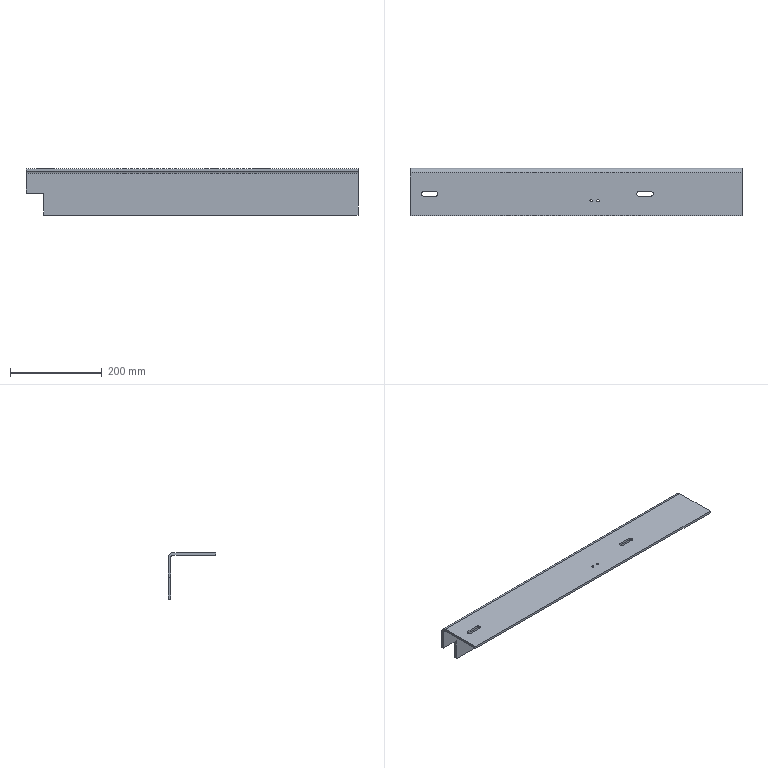Part | NX | 1 solid | 26 faces | box 724.4 x 103.1 x 101 mm | volume 696514 mm3 | plane 14 | cylinder 12 | commonest cylinder face diameters 10 x7 5 x4 20 x1
STEP:
#1=CARTESIAN_POINT('',(671.7,223.9,34.5));
#2=VERTEX_POINT('',#1);
#3=CARTESIAN_POINT('',(671.7,130.8,34.5));
#4=VERTEX_POINT('',#3);
#5=CARTESIAN_POINT('',(671.7,319.307,34.5));
#6=DIRECTION('',(0.,-1.,0.));
#7=VECTOR('',#6,1000.);
#8=LINE('',#5,#7);
#9=EDGE_CURVE('',#2,#4,#8,.T.);
#10=ORIENTED_EDGE('',*,*,#9,.T.);
#11=CARTESIAN_POINT('',(671.7,130.8,29.5));
#12=VERTEX_POINT('',#11);
#13=CARTESIAN_POINT('',(671.7,130.8,29.5));
#14=DIRECTION('',(0.,0.,1.));
#15=VECTOR('',#14,1000.);
#16=LINE('',#13,#15);
#17=EDGE_CURVE('',#12,#4,#16,.T.);
#18=ORIENTED_EDGE('',*,*,#17,.F.);
#19=CARTESIAN_POINT('',(671.7,223.9,29.5));
#20=VERTEX_POINT('',#19);
#21=CARTESIAN_POINT('',(671.7,141.246,29.5));
#22=DIRECTION('',(0.,1.,0.));
#23=VECTOR('',#22,1000.);
#24=LINE('',#21,#23);
#25=EDGE_CURVE('',#12,#20,#24,.T.);
#26=ORIENTED_EDGE('',*,*,#25,.T.);
#27=CARTESIAN_POINT('',(671.7,228.9,24.5));
#28=VERTEX_POINT('',#27);
#29=CARTESIAN_POINT('',(671.7,223.9,24.5));
#30=DIRECTION('',(-1.,0.,0.));
#31=DIRECTION('',(0.,0.,1.));
#32=AXIS2_PLACEMENT_3D('',#29,#30,#31);
#33=CIRCLE('',#32,5.);
#34=EDGE_CURVE('',#20,#28,#33,.T.);
#35=ORIENTED_EDGE('',*,*,#34,.T.);
#36=CARTESIAN_POINT('',(671.7,228.9,-66.5));
#37=VERTEX_POINT('',#36);
#38=CARTESIAN_POINT('',(671.7,228.9,29.5));
#39=DIRECTION('',(0.,0.,-1.));
#40=VECTOR('',#39,1000.);
#41=LINE('',#38,#40);
#42=EDGE_CURVE('',#28,#37,#41,.T.);
#43=ORIENTED_EDGE('',*,*,#42,.T.);
#44=CARTESIAN_POINT('',(671.7,233.9,-66.5));
#45=VERTEX_POINT('',#44);
#46=CARTESIAN_POINT('',(671.7,141.246,-66.5));
#47=DIRECTION('',(0.,1.,0.));
#48=VECTOR('',#47,1000.);
#49=LINE('',#46,#48);
#50=EDGE_CURVE('',#37,#45,#49,.T.);
#51=ORIENTED_EDGE('',*,*,#50,.T.);
#52=CARTESIAN_POINT('',(671.7,233.9,24.5));
#53=VERTEX_POINT('',#52);
#54=CARTESIAN_POINT('',(671.7,233.9,29.5));
#55=DIRECTION('',(0.,0.,1.));
#56=VECTOR('',#55,1000.);
#57=LINE('',#54,#56);
#58=EDGE_CURVE('',#45,#53,#57,.T.);
#59=ORIENTED_EDGE('',*,*,#58,.T.);
#60=CARTESIAN_POINT('',(671.7,223.9,24.5));
#61=DIRECTION('',(1.,0.,0.));
#62=DIRECTION('',(0.,1.,0.));
#63=AXIS2_PLACEMENT_3D('',#60,#61,#62);
#64=CIRCLE('',#63,10.);
#65=EDGE_CURVE('',#53,#2,#64,.T.);
#66=ORIENTED_EDGE('',*,*,#65,.T.);
#67=EDGE_LOOP('',(#10,#18,#26,#35,#43,#51,#59,#66));
#68=FACE_BOUND('',#67,.T.);
#69=CARTESIAN_POINT('',(671.7,165.9,29.5));
#70=DIRECTION('',(1.,0.,0.));
#71=DIRECTION('',(0.,1.,0.));
#72=AXIS2_PLACEMENT_3D('',#69,#70,#71);
#73=PLANE('',#72);
#74=ADVANCED_FACE('',(#68),#73,.T.);
#75=CARTESIAN_POINT('',(-52.7,130.8,29.5));
#76=VERTEX_POINT('',#75);
#77=CARTESIAN_POINT('',(357.184,130.8,29.5));
#78=DIRECTION('',(1.,0.,0.));
#79=VECTOR('',#78,1000.);
#80=LINE('',#77,#79);
#81=EDGE_CURVE('',#76,#12,#80,.T.);
#82=ORIENTED_EDGE('',*,*,#81,.T.);
#83=ORIENTED_EDGE('',*,*,#17,.T.);
#84=CARTESIAN_POINT('',(-52.7,130.8,34.5));
#85=VERTEX_POINT('',#84);
#86=CARTESIAN_POINT('',(357.184,130.8,34.5));
#87=DIRECTION('',(1.,0.,0.));
#88=VECTOR('',#87,1000.);
#89=LINE('',#86,#88);
#90=EDGE_CURVE('',#85,#4,#89,.T.);
#91=ORIENTED_EDGE('',*,*,#90,.F.);
#92=CARTESIAN_POINT('',(-52.7,130.8,29.5));
#93=DIRECTION('',(0.,0.,-1.));
#94=VECTOR('',#93,1000.);
#95=LINE('',#92,#94);
#96=EDGE_CURVE('',#85,#76,#95,.T.);
#97=ORIENTED_EDGE('',*,*,#96,.T.);
#98=EDGE_LOOP('',(#82,#83,#91,#97));
#99=FACE_BOUND('',#98,.T.);
#100=CARTESIAN_POINT('',(364.7,130.8,29.5));
#101=DIRECTION('',(0.,-1.,0.));
#102=DIRECTION('',(0.,0.,-1.));
#103=AXIS2_PLACEMENT_3D('',#100,#101,#102);
#104=PLANE('',#103);
#105=ADVANCED_FACE('',(#99),#104,.T.);
#106=ORIENTED_EDGE('',*,*,#9,.F.);
#107=CARTESIAN_POINT('',(-52.7,223.9,34.5));
#108=VERTEX_POINT('',#107);
#109=CARTESIAN_POINT('',(357.184,223.9,34.5));
#110=DIRECTION('',(1.,0.,0.));
#111=VECTOR('',#110,1000.);
#112=LINE('',#109,#111);
#113=EDGE_CURVE('',#108,#2,#112,.T.);
#114=ORIENTED_EDGE('',*,*,#113,.F.);
#115=CARTESIAN_POINT('',(-52.7,233.9,34.5));
#116=DIRECTION('',(0.,1.,0.));
#117=VECTOR('',#116,1000.);
#118=LINE('',#115,#117);
#119=EDGE_CURVE('',#85,#108,#118,.T.);
#120=ORIENTED_EDGE('',*,*,#119,.F.);
#121=ORIENTED_EDGE('',*,*,#90,.T.);
#122=EDGE_LOOP('',(#106,#114,#120,#121));
#123=FACE_BOUND('',#122,.T.);
#124=CARTESIAN_POINT('',(340.,163.7,34.5));
#125=VERTEX_POINT('',#124);
#126=CARTESIAN_POINT('',(345.,163.7,34.5));
#127=VERTEX_POINT('',#126);
#128=CARTESIAN_POINT('',(342.5,163.7,34.5));
#129=DIRECTION('',(0.,0.,1.));
#130=DIRECTION('',(1.,0.,0.));
#131=AXIS2_PLACEMENT_3D('',#128,#129,#130);
#132=CIRCLE('',#131,2.5);
#133=EDGE_CURVE('',#125,#127,#132,.T.);
#134=ORIENTED_EDGE('',*,*,#133,.F.);
#135=CARTESIAN_POINT('',(342.5,163.7,34.5));
#136=DIRECTION('',(0.,0.,1.));
#137=DIRECTION('',(1.,0.,0.));
#138=AXIS2_PLACEMENT_3D('',#135,#136,#137);
#139=CIRCLE('',#138,2.5);
#140=EDGE_CURVE('',#127,#125,#139,.T.);
#141=ORIENTED_EDGE('',*,*,#140,.F.);
#142=EDGE_LOOP('',(#134,#141));
#143=FACE_BOUND('',#142,.T.);
#144=CARTESIAN_POINT('',(355.,163.7,34.5));
#145=VERTEX_POINT('',#144);
#146=CARTESIAN_POINT('',(360.,163.7,34.5));
#147=VERTEX_POINT('',#146);
#148=CARTESIAN_POINT('',(357.5,163.7,34.5));
#149=DIRECTION('',(0.,0.,1.));
#150=DIRECTION('',(1.,0.,0.));
#151=AXIS2_PLACEMENT_3D('',#148,#149,#150);
#152=CIRCLE('',#151,2.5);
#153=EDGE_CURVE('',#145,#147,#152,.T.);
#154=ORIENTED_EDGE('',*,*,#153,.F.);
#155=CARTESIAN_POINT('',(357.5,163.7,34.5));
#156=DIRECTION('',(0.,0.,1.));
#157=DIRECTION('',(1.,0.,0.));
#158=AXIS2_PLACEMENT_3D('',#155,#156,#157);
#159=CIRCLE('',#158,2.5);
#160=EDGE_CURVE('',#147,#145,#159,.T.);
#161=ORIENTED_EDGE('',*,*,#160,.F.);
#162=EDGE_LOOP('',(#154,#161));
#163=FACE_BOUND('',#162,.T.);
#164=CARTESIAN_POINT('',(3.125,173.2,34.5));
#165=VERTEX_POINT('',#164);
#166=CARTESIAN_POINT('',(8.125,178.2,34.5));
#167=VERTEX_POINT('',#166);
#168=CARTESIAN_POINT('',(3.125,178.2,34.5));
#169=DIRECTION('',(0.,0.,1.));
#170=DIRECTION('',(1.,0.,0.));
#171=AXIS2_PLACEMENT_3D('',#168,#169,#170);
#172=CIRCLE('',#171,5.);
#173=EDGE_CURVE('',#165,#167,#172,.T.);
#174=ORIENTED_EDGE('',*,*,#173,.F.);
#175=CARTESIAN_POINT('',(-23.125,173.2,34.5));
#176=VERTEX_POINT('',#175);
#177=CARTESIAN_POINT('',(357.184,173.2,34.5));
#178=DIRECTION('',(1.,0.,0.));
#179=VECTOR('',#178,1000.);
#180=LINE('',#177,#179);
#181=EDGE_CURVE('',#176,#165,#180,.T.);
#182=ORIENTED_EDGE('',*,*,#181,.F.);
#183=CARTESIAN_POINT('',(-23.125,183.2,34.5));
#184=VERTEX_POINT('',#183);
#185=CARTESIAN_POINT('',(-23.125,178.2,34.5));
#186=DIRECTION('',(0.,0.,1.));
#187=DIRECTION('',(1.,0.,0.));
#188=AXIS2_PLACEMENT_3D('',#185,#186,#187);
#189=CIRCLE('',#188,5.);
#190=EDGE_CURVE('',#184,#176,#189,.T.);
#191=ORIENTED_EDGE('',*,*,#190,.F.);
#192=CARTESIAN_POINT('',(3.125,183.2,34.5));
#193=VERTEX_POINT('',#192);
#194=CARTESIAN_POINT('',(357.184,183.2,34.5));
#195=DIRECTION('',(-1.,0.,0.));
#196=VECTOR('',#195,1000.);
#197=LINE('',#194,#196);
#198=EDGE_CURVE('',#193,#184,#197,.T.);
#199=ORIENTED_EDGE('',*,*,#198,.F.);
#200=CARTESIAN_POINT('',(3.125,178.2,34.5));
#201=DIRECTION('',(0.,0.,1.));
#202=DIRECTION('',(1.,0.,0.));
#203=AXIS2_PLACEMENT_3D('',#200,#201,#202);
#204=CIRCLE('',#203,5.);
#205=EDGE_CURVE('',#167,#193,#204,.T.);
#206=ORIENTED_EDGE('',*,*,#205,.F.);
#207=EDGE_LOOP('',(#174,#182,#191,#199,#206));
#208=FACE_BOUND('',#207,.T.);
#209=CARTESIAN_POINT('',(473.125,173.2,34.5));
#210=VERTEX_POINT('',#209);
#211=CARTESIAN_POINT('',(478.125,178.2,34.5));
#212=VERTEX_POINT('',#211);
#213=CARTESIAN_POINT('',(473.125,178.2,34.5));
#214=DIRECTION('',(0.,0.,1.));
#215=DIRECTION('',(1.,0.,0.));
#216=AXIS2_PLACEMENT_3D('',#213,#214,#215);
#217=CIRCLE('',#216,5.);
#218=EDGE_CURVE('',#210,#212,#217,.T.);
#219=ORIENTED_EDGE('',*,*,#218,.F.);
#220=CARTESIAN_POINT('',(446.875,173.2,34.5));
#221=VERTEX_POINT('',#220);
#222=CARTESIAN_POINT('',(357.184,173.2,34.5));
#223=DIRECTION('',(1.,0.,0.));
#224=VECTOR('',#223,1000.);
#225=LINE('',#222,#224);
#226=EDGE_CURVE('',#221,#210,#225,.T.);
#227=ORIENTED_EDGE('',*,*,#226,.F.);
#228=CARTESIAN_POINT('',(446.875,183.2,34.5));
#229=VERTEX_POINT('',#228);
#230=CARTESIAN_POINT('',(446.875,178.2,34.5));
#231=DIRECTION('',(0.,0.,1.));
#232=DIRECTION('',(1.,0.,0.));
#233=AXIS2_PLACEMENT_3D('',#230,#231,#232);
#234=CIRCLE('',#233,5.);
#235=EDGE_CURVE('',#229,#221,#234,.T.);
#236=ORIENTED_EDGE('',*,*,#235,.F.);
#237=CARTESIAN_POINT('',(473.125,183.2,34.5));
#238=VERTEX_POINT('',#237);
#239=CARTESIAN_POINT('',(357.184,183.2,34.5));
#240=DIRECTION('',(-1.,0.,0.));
#241=VECTOR('',#240,1000.);
#242=LINE('',#239,#241);
#243=EDGE_CURVE('',#238,#229,#242,.T.);
#244=ORIENTED_EDGE('',*,*,#243,.F.);
#245=CARTESIAN_POINT('',(473.125,178.2,34.5));
#246=DIRECTION('',(0.,0.,1.));
#247=DIRECTION('',(1.,0.,0.));
#248=AXIS2_PLACEMENT_3D('',#245,#246,#247);
#249=CIRCLE('',#248,5.);
#250=EDGE_CURVE('',#212,#238,#249,.T.);
#251=ORIENTED_EDGE('',*,*,#250,.F.);
#252=EDGE_LOOP('',(#219,#227,#236,#244,#251));
#253=FACE_BOUND('',#252,.T.);
#254=CARTESIAN_POINT('',(-52.7,233.9,34.5));
#255=DIRECTION('',(0.,0.,1.));
#256=DIRECTION('',(1.,0.,0.));
#257=AXIS2_PLACEMENT_3D('',#254,#255,#256);
#258=PLANE('',#257);
#259=ADVANCED_FACE('',(#123,#143,#163,#208,#253),#258,.T.);
#260=CARTESIAN_POINT('',(-52.7,228.9,-18.5));
#261=VERTEX_POINT('',#260);
#262=CARTESIAN_POINT('',(-52.7,233.9,-18.5));
#263=VERTEX_POINT('',#262);
#264=CARTESIAN_POINT('',(-52.7,141.246,-18.5));
#265=DIRECTION('',(0.,1.,0.));
#266=VECTOR('',#265,1000.);
#267=LINE('',#264,#266);
#268=EDGE_CURVE('',#261,#263,#267,.T.);
#269=ORIENTED_EDGE('',*,*,#268,.F.);
#270=CARTESIAN_POINT('',(-52.7,228.9,24.5));
#271=VERTEX_POINT('',#270);
#272=CARTESIAN_POINT('',(-52.7,228.9,29.5));
#273=DIRECTION('',(0.,0.,1.));
#274=VECTOR('',#273,1000.);
#275=LINE('',#272,#274);
#276=EDGE_CURVE('',#261,#271,#275,.T.);
#277=ORIENTED_EDGE('',*,*,#276,.T.);
#278=CARTESIAN_POINT('',(-52.7,223.9,29.5));
#279=VERTEX_POINT('',#278);
#280=CARTESIAN_POINT('',(-52.7,223.9,24.5));
#281=DIRECTION('',(1.,0.,0.));
#282=DIRECTION('',(0.,1.,0.));
#283=AXIS2_PLACEMENT_3D('',#280,#281,#282);
#284=CIRCLE('',#283,5.);
#285=EDGE_CURVE('',#271,#279,#284,.T.);
#286=ORIENTED_EDGE('',*,*,#285,.T.);
#287=CARTESIAN_POINT('',(-52.7,141.246,29.5));
#288=DIRECTION('',(0.,-1.,0.));
#289=VECTOR('',#288,1000.);
#290=LINE('',#287,#289);
#291=EDGE_CURVE('',#279,#76,#290,.T.);
#292=ORIENTED_EDGE('',*,*,#291,.T.);
#293=ORIENTED_EDGE('',*,*,#96,.F.);
#294=ORIENTED_EDGE('',*,*,#119,.T.);
#295=CARTESIAN_POINT('',(-52.7,233.9,24.5));
#296=VERTEX_POINT('',#295);
#297=CARTESIAN_POINT('',(-52.7,223.9,24.5));
#298=DIRECTION('',(-1.,0.,0.));
#299=DIRECTION('',(0.,0.,1.));
#300=AXIS2_PLACEMENT_3D('',#297,#298,#299);
#301=CIRCLE('',#300,10.);
#302=EDGE_CURVE('',#108,#296,#301,.T.);
#303=ORIENTED_EDGE('',*,*,#302,.T.);
#304=CARTESIAN_POINT('',(-52.7,233.9,29.5));
#305=DIRECTION('',(0.,0.,-1.));
#306=VECTOR('',#305,1000.);
#307=LINE('',#304,#306);
#308=EDGE_CURVE('',#296,#263,#307,.T.);
#309=ORIENTED_EDGE('',*,*,#308,.T.);
#310=EDGE_LOOP('',(#269,#277,#286,#292,#293,#294,#303,#309));
#311=FACE_BOUND('',#310,.T.);
#312=CARTESIAN_POINT('',(-52.7,233.9,-60.5));
#313=DIRECTION('',(-1.,0.,0.));
#314=DIRECTION('',(0.,0.,1.));
#315=AXIS2_PLACEMENT_3D('',#312,#313,#314);
#316=PLANE('',#315);
#317=ADVANCED_FACE('',(#311),#316,.T.);
#318=CARTESIAN_POINT('',(-13.7,233.9,-66.5));
#319=VERTEX_POINT('',#318);
#320=CARTESIAN_POINT('',(-13.7,228.9,-66.5));
#321=VERTEX_POINT('',#320);
#322=CARTESIAN_POINT('',(-13.7,141.246,-66.5));
#323=DIRECTION('',(0.,-1.,0.));
#324=VECTOR('',#323,1000.);
#325=LINE('',#322,#324);
#326=EDGE_CURVE('',#319,#321,#325,.T.);
#327=ORIENTED_EDGE('',*,*,#326,.F.);
#328=CARTESIAN_POINT('',(357.184,233.9,-66.5));
#329=DIRECTION('',(-1.,0.,0.));
#330=VECTOR('',#329,1000.);
#331=LINE('',#328,#330);
#332=EDGE_CURVE('',#45,#319,#331,.T.);
#333=ORIENTED_EDGE('',*,*,#332,.F.);
#334=ORIENTED_EDGE('',*,*,#50,.F.);
#335=CARTESIAN_POINT('',(357.184,228.9,-66.5));
#336=DIRECTION('',(-1.,0.,0.));
#337=VECTOR('',#336,1000.);
#338=LINE('',#335,#337);
#339=EDGE_CURVE('',#37,#321,#338,.T.);
#340=ORIENTED_EDGE('',*,*,#339,.T.);
#341=EDGE_LOOP('',(#327,#333,#334,#340));
#342=FACE_BOUND('',#341,.T.);
#343=CARTESIAN_POINT('',(671.7,233.9,-66.5));
#344=DIRECTION('',(0.,0.,-1.));
#345=DIRECTION('',(0.,-1.,0.));
#346=AXIS2_PLACEMENT_3D('',#343,#344,#345);
#347=PLANE('',#346);
#348=ADVANCED_FACE('',(#342),#347,.T.);
#349=CARTESIAN_POINT('',(357.184,233.9,24.5));
#350=DIRECTION('',(1.,0.,0.));
#351=VECTOR('',#350,1000.);
#352=LINE('',#349,#351);
#353=EDGE_CURVE('',#296,#53,#352,.T.);
#354=ORIENTED_EDGE('',*,*,#353,.T.);
#355=ORIENTED_EDGE('',*,*,#58,.F.);
#356=ORIENTED_EDGE('',*,*,#332,.T.);
#357=CARTESIAN_POINT('',(-13.7,233.9,-18.5));
#358=VERTEX_POINT('',#357);
#359=CARTESIAN_POINT('',(-13.7,233.9,29.5));
#360=DIRECTION('',(0.,0.,-1.));
#361=VECTOR('',#360,1000.);
#362=LINE('',#359,#361);
#363=EDGE_CURVE('',#358,#319,#362,.T.);
#364=ORIENTED_EDGE('',*,*,#363,.F.);
#365=CARTESIAN_POINT('',(357.184,233.9,-18.5));
#366=DIRECTION('',(1.,0.,0.));
#367=VECTOR('',#366,1000.);
#368=LINE('',#365,#367);
#369=EDGE_CURVE('',#263,#358,#368,.T.);
#370=ORIENTED_EDGE('',*,*,#369,.F.);
#371=ORIENTED_EDGE('',*,*,#308,.F.);
#372=EDGE_LOOP('',(#354,#355,#356,#364,#370,#371));
#373=FACE_BOUND('',#372,.T.);
#374=CARTESIAN_POINT('',(-52.7,233.9,24.907));
#375=DIRECTION('',(0.,1.,0.));
#376=DIRECTION('',(1.,0.,0.));
#377=AXIS2_PLACEMENT_3D('',#374,#375,#376);
#378=PLANE('',#377);
#379=ADVANCED_FACE('',(#373),#378,.T.);
#380=ORIENTED_EDGE('',*,*,#113,.T.);
#381=ORIENTED_EDGE('',*,*,#65,.F.);
#382=ORIENTED_EDGE('',*,*,#353,.F.);
#383=ORIENTED_EDGE('',*,*,#302,.F.);
#384=EDGE_LOOP('',(#380,#381,#382,#383));
#385=FACE_BOUND('',#384,.T.);
#386=CARTESIAN_POINT('',(671.7,223.9,24.5));
#387=DIRECTION('',(1.,0.,0.));
#388=DIRECTION('',(0.,-1.,0.));
#389=AXIS2_PLACEMENT_3D('',#386,#387,#388);
#390=CYLINDRICAL_SURFACE('',#389,10.);
#391=ADVANCED_FACE('',(#385),#390,.T.);
#392=ORIENTED_EDGE('',*,*,#133,.T.);
#393=CARTESIAN_POINT('',(345.,163.7,29.5));
#394=VERTEX_POINT('',#393);
#395=CARTESIAN_POINT('',(345.,163.7,34.5));
#396=DIRECTION('',(0.,0.,1.));
#397=VECTOR('',#396,1000.);
#398=LINE('',#395,#397);
#399=EDGE_CURVE('',#394,#127,#398,.T.);
#400=ORIENTED_EDGE('',*,*,#399,.F.);
#401=CARTESIAN_POINT('',(340.,163.7,29.5));
#402=VERTEX_POINT('',#401);
#403=CARTESIAN_POINT('',(342.5,163.7,29.5));
#404=DIRECTION('',(0.,0.,1.));
#405=DIRECTION('',(1.,0.,0.));
#406=AXIS2_PLACEMENT_3D('',#403,#404,#405);
#407=CIRCLE('',#406,2.5);
#408=EDGE_CURVE('',#402,#394,#407,.T.);
#409=ORIENTED_EDGE('',*,*,#408,.F.);
#410=CARTESIAN_POINT('',(340.,163.7,34.5));
#411=DIRECTION('',(0.,0.,1.));
#412=VECTOR('',#411,1000.);
#413=LINE('',#410,#412);
#414=EDGE_CURVE('',#402,#125,#413,.T.);
#415=ORIENTED_EDGE('',*,*,#414,.T.);
#416=EDGE_LOOP('',(#392,#400,#409,#415));
#417=FACE_BOUND('',#416,.T.);
#418=CARTESIAN_POINT('',(342.5,163.7,34.5));
#419=DIRECTION('',(0.,0.,1.));
#420=DIRECTION('',(1.,0.,0.));
#421=AXIS2_PLACEMENT_3D('',#418,#419,#420);
#422=CYLINDRICAL_SURFACE('',#421,2.5);
#423=ADVANCED_FACE('',(#417),#422,.F.);
#424=CARTESIAN_POINT('',(-13.7,228.9,-18.5));
#425=VERTEX_POINT('',#424);
#426=CARTESIAN_POINT('',(357.184,228.9,-18.5));
#427=DIRECTION('',(1.,0.,0.));
#428=VECTOR('',#427,1000.);
#429=LINE('',#426,#428);
#430=EDGE_CURVE('',#261,#425,#429,.T.);
#431=ORIENTED_EDGE('',*,*,#430,.F.);
#432=ORIENTED_EDGE('',*,*,#268,.T.);
#433=ORIENTED_EDGE('',*,*,#369,.T.);
#434=CARTESIAN_POINT('',(-13.7,141.246,-18.5));
#435=DIRECTION('',(0.,1.,0.));
#436=VECTOR('',#435,1000.);
#437=LINE('',#434,#436);
#438=EDGE_CURVE('',#425,#358,#437,.T.);
#439=ORIENTED_EDGE('',*,*,#438,.F.);
#440=EDGE_LOOP('',(#431,#432,#433,#439));
#441=FACE_BOUND('',#440,.T.);
#442=CARTESIAN_POINT('',(-10.7,120.49,-18.5));
#443=DIRECTION('',(0.,0.,1.));
#444=DIRECTION('',(1.,0.,0.));
#445=AXIS2_PLACEMENT_3D('',#442,#443,#444);
#446=PLANE('',#445);
#447=ADVANCED_FACE('',(#441),#446,.F.);
#448=ORIENTED_EDGE('',*,*,#363,.T.);
#449=ORIENTED_EDGE('',*,*,#326,.T.);
#450=CARTESIAN_POINT('',(-13.7,228.9,29.5));
#451=DIRECTION('',(0.,0.,-1.));
#452=VECTOR('',#451,1000.);
#453=LINE('',#450,#452);
#454=EDGE_CURVE('',#425,#321,#453,.T.);
#455=ORIENTED_EDGE('',*,*,#454,.F.);
#456=ORIENTED_EDGE('',*,*,#438,.T.);
#457=EDGE_LOOP('',(#448,#449,#455,#456));
#458=FACE_BOUND('',#457,.T.);
#459=CARTESIAN_POINT('',(-13.7,120.49,-66.5));
#460=DIRECTION('',(1.,0.,0.));
#461=DIRECTION('',(0.,1.,0.));
#462=AXIS2_PLACEMENT_3D('',#459,#460,#461);
#463=PLANE('',#462);
#464=ADVANCED_FACE('',(#458),#463,.F.);
#465=ORIENTED_EDGE('',*,*,#399,.T.);
#466=ORIENTED_EDGE('',*,*,#140,.T.);
#467=ORIENTED_EDGE('',*,*,#414,.F.);
#468=CARTESIAN_POINT('',(342.5,163.7,29.5));
#469=DIRECTION('',(0.,0.,1.));
#470=DIRECTION('',(1.,0.,0.));
#471=AXIS2_PLACEMENT_3D('',#468,#469,#470);
#472=CIRCLE('',#471,2.5);
#473=EDGE_CURVE('',#394,#402,#472,.T.);
#474=ORIENTED_EDGE('',*,*,#473,.F.);
#475=EDGE_LOOP('',(#465,#466,#467,#474));
#476=FACE_BOUND('',#475,.T.);
#477=CARTESIAN_POINT('',(342.5,163.7,34.5));
#478=DIRECTION('',(0.,0.,1.));
#479=DIRECTION('',(1.,0.,0.));
#480=AXIS2_PLACEMENT_3D('',#477,#478,#479);
#481=CYLINDRICAL_SURFACE('',#480,2.5);
#482=ADVANCED_FACE('',(#476),#481,.F.);
#483=ORIENTED_EDGE('',*,*,#42,.F.);
#484=CARTESIAN_POINT('',(357.184,228.9,24.5));
#485=DIRECTION('',(1.,0.,0.));
#486=VECTOR('',#485,1000.);
#487=LINE('',#484,#486);
#488=EDGE_CURVE('',#271,#28,#487,.T.);
#489=ORIENTED_EDGE('',*,*,#488,.F.);
#490=ORIENTED_EDGE('',*,*,#276,.F.);
#491=ORIENTED_EDGE('',*,*,#430,.T.);
#492=ORIENTED_EDGE('',*,*,#454,.T.);
#493=ORIENTED_EDGE('',*,*,#339,.F.);
#494=EDGE_LOOP('',(#483,#489,#490,#491,#492,#493));
#495=FACE_BOUND('',#494,.T.);
#496=CARTESIAN_POINT('',(357.184,228.9,117.561));
#497=DIRECTION('',(0.,1.,0.));
#498=DIRECTION('',(1.,0.,0.));
#499=AXIS2_PLACEMENT_3D('',#496,#497,#498);
#500=PLANE('',#499);
#501=ADVANCED_FACE('',(#495),#500,.F.);
#502=CARTESIAN_POINT('',(357.184,223.9,29.5));
#503=DIRECTION('',(1.,0.,0.));
#504=VECTOR('',#503,1000.);
#505=LINE('',#502,#504);
#506=EDGE_CURVE('',#279,#20,#505,.T.);
#507=ORIENTED_EDGE('',*,*,#506,.T.);
#508=ORIENTED_EDGE('',*,*,#25,.F.);
#509=ORIENTED_EDGE('',*,*,#81,.F.);
#510=ORIENTED_EDGE('',*,*,#291,.F.);
#511=EDGE_LOOP('',(#507,#508,#509,#510));
#512=FACE_BOUND('',#511,.T.);
#513=ORIENTED_EDGE('',*,*,#408,.T.);
#514=ORIENTED_EDGE('',*,*,#473,.T.);
#515=EDGE_LOOP('',(#513,#514));
#516=FACE_BOUND('',#515,.T.);
#517=CARTESIAN_POINT('',(355.,163.7,29.5));
#518=VERTEX_POINT('',#517);
#519=CARTESIAN_POINT('',(360.,163.7,29.5));
#520=VERTEX_POINT('',#519);
#521=CARTESIAN_POINT('',(357.5,163.7,29.5));
#522=DIRECTION('',(0.,0.,1.));
#523=DIRECTION('',(1.,0.,0.));
#524=AXIS2_PLACEMENT_3D('',#521,#522,#523);
#525=CIRCLE('',#524,2.5);
#526=EDGE_CURVE('',#518,#520,#525,.T.);
#527=ORIENTED_EDGE('',*,*,#526,.T.);
#528=CARTESIAN_POINT('',(357.5,163.7,29.5));
#529=DIRECTION('',(0.,0.,1.));
#530=DIRECTION('',(1.,0.,0.));
#531=AXIS2_PLACEMENT_3D('',#528,#529,#530);
#532=CIRCLE('',#531,2.5);
#533=EDGE_CURVE('',#520,#518,#532,.T.);
#534=ORIENTED_EDGE('',*,*,#533,.T.);
#535=EDGE_LOOP('',(#527,#534));
#536=FACE_BOUND('',#535,.T.);
#537=CARTESIAN_POINT('',(3.125,183.2,29.5));
#538=VERTEX_POINT('',#537);
#539=CARTESIAN_POINT('',(-23.125,183.2,29.5));
#540=VERTEX_POINT('',#539);
#541=CARTESIAN_POINT('',(357.184,183.2,29.5));
#542=DIRECTION('',(-1.,0.,0.));
#543=VECTOR('',#542,1000.);
#544=LINE('',#541,#543);
#545=EDGE_CURVE('',#538,#540,#544,.T.);
#546=ORIENTED_EDGE('',*,*,#545,.T.);
#547=CARTESIAN_POINT('',(-23.125,173.2,29.5));
#548=VERTEX_POINT('',#547);
#549=CARTESIAN_POINT('',(-23.125,178.2,29.5));
#550=DIRECTION('',(0.,0.,1.));
#551=DIRECTION('',(1.,0.,0.));
#552=AXIS2_PLACEMENT_3D('',#549,#550,#551);
#553=CIRCLE('',#552,5.);
#554=EDGE_CURVE('',#540,#548,#553,.T.);
#555=ORIENTED_EDGE('',*,*,#554,.T.);
#556=CARTESIAN_POINT('',(3.125,173.2,29.5));
#557=VERTEX_POINT('',#556);
#558=CARTESIAN_POINT('',(357.184,173.2,29.5));
#559=DIRECTION('',(1.,0.,0.));
#560=VECTOR('',#559,1000.);
#561=LINE('',#558,#560);
#562=EDGE_CURVE('',#548,#557,#561,.T.);
#563=ORIENTED_EDGE('',*,*,#562,.T.);
#564=CARTESIAN_POINT('',(8.125,178.2,29.5));
#565=VERTEX_POINT('',#564);
#566=CARTESIAN_POINT('',(3.125,178.2,29.5));
#567=DIRECTION('',(0.,0.,1.));
#568=DIRECTION('',(1.,0.,0.));
#569=AXIS2_PLACEMENT_3D('',#566,#567,#568);
#570=CIRCLE('',#569,5.);
#571=EDGE_CURVE('',#557,#565,#570,.T.);
#572=ORIENTED_EDGE('',*,*,#571,.T.);
#573=CARTESIAN_POINT('',(3.125,178.2,29.5));
#574=DIRECTION('',(0.,0.,1.));
#575=DIRECTION('',(1.,0.,0.));
#576=AXIS2_PLACEMENT_3D('',#573,#574,#575);
#577=CIRCLE('',#576,5.);
#578=EDGE_CURVE('',#565,#538,#577,.T.);
#579=ORIENTED_EDGE('',*,*,#578,.T.);
#580=EDGE_LOOP('',(#546,#555,#563,#572,#579));
#581=FACE_BOUND('',#580,.T.);
#582=CARTESIAN_POINT('',(473.125,173.2,29.5));
#583=VERTEX_POINT('',#582);
#584=CARTESIAN_POINT('',(478.125,178.2,29.5));
#585=VERTEX_POINT('',#584);
#586=CARTESIAN_POINT('',(473.125,178.2,29.5));
#587=DIRECTION('',(0.,0.,1.));
#588=DIRECTION('',(1.,0.,0.));
#589=AXIS2_PLACEMENT_3D('',#586,#587,#588);
#590=CIRCLE('',#589,5.);
#591=EDGE_CURVE('',#583,#585,#590,.T.);
#592=ORIENTED_EDGE('',*,*,#591,.T.);
#593=CARTESIAN_POINT('',(473.125,183.2,29.5));
#594=VERTEX_POINT('',#593);
#595=CARTESIAN_POINT('',(473.125,178.2,29.5));
#596=DIRECTION('',(0.,0.,1.));
#597=DIRECTION('',(1.,0.,0.));
#598=AXIS2_PLACEMENT_3D('',#595,#596,#597);
#599=CIRCLE('',#598,5.);
#600=EDGE_CURVE('',#585,#594,#599,.T.);
#601=ORIENTED_EDGE('',*,*,#600,.T.);
#602=CARTESIAN_POINT('',(446.875,183.2,29.5));
#603=VERTEX_POINT('',#602);
#604=CARTESIAN_POINT('',(357.184,183.2,29.5));
#605=DIRECTION('',(-1.,0.,0.));
#606=VECTOR('',#605,1000.);
#607=LINE('',#604,#606);
#608=EDGE_CURVE('',#594,#603,#607,.T.);
#609=ORIENTED_EDGE('',*,*,#608,.T.);
#610=CARTESIAN_POINT('',(446.875,173.2,29.5));
#611=VERTEX_POINT('',#610);
#612=CARTESIAN_POINT('',(446.875,178.2,29.5));
#613=DIRECTION('',(0.,0.,1.));
#614=DIRECTION('',(1.,0.,0.));
#615=AXIS2_PLACEMENT_3D('',#612,#613,#614);
#616=CIRCLE('',#615,5.);
#617=EDGE_CURVE('',#603,#611,#616,.T.);
#618=ORIENTED_EDGE('',*,*,#617,.T.);
#619=CARTESIAN_POINT('',(357.184,173.2,29.5));
#620=DIRECTION('',(1.,0.,0.));
#621=VECTOR('',#620,1000.);
#622=LINE('',#619,#621);
#623=EDGE_CURVE('',#611,#583,#622,.T.);
#624=ORIENTED_EDGE('',*,*,#623,.T.);
#625=EDGE_LOOP('',(#592,#601,#609,#618,#624));
#626=FACE_BOUND('',#625,.T.);
#627=CARTESIAN_POINT('',(357.184,141.246,29.5));
#628=DIRECTION('',(0.,0.,1.));
#629=DIRECTION('',(1.,0.,0.));
#630=AXIS2_PLACEMENT_3D('',#627,#628,#629);
#631=PLANE('',#630);
#632=ADVANCED_FACE('',(#512,#516,#536,#581,#626),#631,.F.);
#633=ORIENTED_EDGE('',*,*,#488,.T.);
#634=ORIENTED_EDGE('',*,*,#34,.F.);
#635=ORIENTED_EDGE('',*,*,#506,.F.);
#636=ORIENTED_EDGE('',*,*,#285,.F.);
#637=EDGE_LOOP('',(#633,#634,#635,#636));
#638=FACE_BOUND('',#637,.T.);
#639=CARTESIAN_POINT('',(671.7,223.9,24.5));
#640=DIRECTION('',(1.,0.,0.));
#641=DIRECTION('',(0.,-1.,0.));
#642=AXIS2_PLACEMENT_3D('',#639,#640,#641);
#643=CYLINDRICAL_SURFACE('',#642,5.);
#644=ADVANCED_FACE('',(#638),#643,.F.);
#645=ORIENTED_EDGE('',*,*,#153,.T.);
#646=CARTESIAN_POINT('',(360.,163.7,34.5));
#647=DIRECTION('',(0.,0.,1.));
#648=VECTOR('',#647,1000.);
#649=LINE('',#646,#648);
#650=EDGE_CURVE('',#520,#147,#649,.T.);
#651=ORIENTED_EDGE('',*,*,#650,.F.);
#652=ORIENTED_EDGE('',*,*,#526,.F.);
#653=CARTESIAN_POINT('',(355.,163.7,34.5));
#654=DIRECTION('',(0.,0.,1.));
#655=VECTOR('',#654,1000.);
#656=LINE('',#653,#655);
#657=EDGE_CURVE('',#518,#145,#656,.T.);
#658=ORIENTED_EDGE('',*,*,#657,.T.);
#659=EDGE_LOOP('',(#645,#651,#652,#658));
#660=FACE_BOUND('',#659,.T.);
#661=CARTESIAN_POINT('',(357.5,163.7,34.5));
#662=DIRECTION('',(0.,0.,1.));
#663=DIRECTION('',(1.,0.,0.));
#664=AXIS2_PLACEMENT_3D('',#661,#662,#663);
#665=CYLINDRICAL_SURFACE('',#664,2.5);
#666=ADVANCED_FACE('',(#660),#665,.F.);
#667=ORIENTED_EDGE('',*,*,#545,.F.);
#668=CARTESIAN_POINT('',(3.125,183.2,-76.6));
#669=DIRECTION('',(0.,0.,1.));
#670=VECTOR('',#669,1000.);
#671=LINE('',#668,#670);
#672=EDGE_CURVE('',#538,#193,#671,.T.);
#673=ORIENTED_EDGE('',*,*,#672,.T.);
#674=ORIENTED_EDGE('',*,*,#198,.T.);
#675=CARTESIAN_POINT('',(-23.125,183.2,-76.6));
#676=DIRECTION('',(0.,0.,1.));
#677=VECTOR('',#676,1000.);
#678=LINE('',#675,#677);
#679=EDGE_CURVE('',#540,#184,#678,.T.);
#680=ORIENTED_EDGE('',*,*,#679,.F.);
#681=EDGE_LOOP('',(#667,#673,#674,#680));
#682=FACE_BOUND('',#681,.T.);
#683=CARTESIAN_POINT('',(-23.125,183.2,-76.6));
#684=DIRECTION('',(0.,1.,0.));
#685=DIRECTION('',(1.,0.,0.));
#686=AXIS2_PLACEMENT_3D('',#683,#684,#685);
#687=PLANE('',#686);
#688=ADVANCED_FACE('',(#682),#687,.F.);
#689=ORIENTED_EDGE('',*,*,#181,.T.);
#690=CARTESIAN_POINT('',(3.125,173.2,-76.6));
#691=DIRECTION('',(0.,0.,1.));
#692=VECTOR('',#691,1000.);
#693=LINE('',#690,#692);
#694=EDGE_CURVE('',#557,#165,#693,.T.);
#695=ORIENTED_EDGE('',*,*,#694,.F.);
#696=ORIENTED_EDGE('',*,*,#562,.F.);
#697=CARTESIAN_POINT('',(-23.125,173.2,-76.6));
#698=DIRECTION('',(0.,0.,1.));
#699=VECTOR('',#698,1000.);
#700=LINE('',#697,#699);
#701=EDGE_CURVE('',#548,#176,#700,.T.);
#702=ORIENTED_EDGE('',*,*,#701,.T.);
#703=EDGE_LOOP('',(#689,#695,#696,#702));
#704=FACE_BOUND('',#703,.T.);
#705=CARTESIAN_POINT('',(3.125,173.2,-76.6));
#706=DIRECTION('',(0.,-1.,0.));
#707=DIRECTION('',(0.,0.,-1.));
#708=AXIS2_PLACEMENT_3D('',#705,#706,#707);
#709=PLANE('',#708);
#710=ADVANCED_FACE('',(#704),#709,.F.);
#711=CARTESIAN_POINT('',(8.125,178.2,-76.6));
#712=DIRECTION('',(0.,0.,1.));
#713=VECTOR('',#712,1000.);
#714=LINE('',#711,#713);
#715=EDGE_CURVE('',#565,#167,#714,.T.);
#716=ORIENTED_EDGE('',*,*,#715,.F.);
#717=ORIENTED_EDGE('',*,*,#571,.F.);
#718=ORIENTED_EDGE('',*,*,#694,.T.);
#719=ORIENTED_EDGE('',*,*,#173,.T.);
#720=EDGE_LOOP('',(#716,#717,#718,#719));
#721=FACE_BOUND('',#720,.T.);
#722=CARTESIAN_POINT('',(3.125,178.2,-76.6));
#723=DIRECTION('',(0.,0.,1.));
#724=DIRECTION('',(1.,0.,0.));
#725=AXIS2_PLACEMENT_3D('',#722,#723,#724);
#726=CYLINDRICAL_SURFACE('',#725,5.);
#727=ADVANCED_FACE('',(#721),#726,.F.);
#728=ORIENTED_EDGE('',*,*,#554,.F.);
#729=ORIENTED_EDGE('',*,*,#679,.T.);
#730=ORIENTED_EDGE('',*,*,#190,.T.);
#731=ORIENTED_EDGE('',*,*,#701,.F.);
#732=EDGE_LOOP('',(#728,#729,#730,#731));
#733=FACE_BOUND('',#732,.T.);
#734=CARTESIAN_POINT('',(-23.125,178.2,-76.6));
#735=DIRECTION('',(0.,0.,1.));
#736=DIRECTION('',(1.,0.,0.));
#737=AXIS2_PLACEMENT_3D('',#734,#735,#736);
#738=CYLINDRICAL_SURFACE('',#737,5.);
#739=ADVANCED_FACE('',(#733),#738,.F.);
#740=ORIENTED_EDGE('',*,*,#617,.F.);
#741=CARTESIAN_POINT('',(446.875,183.2,-76.6));
#742=DIRECTION('',(0.,0.,1.));
#743=VECTOR('',#742,1000.);
#744=LINE('',#741,#743);
#745=EDGE_CURVE('',#603,#229,#744,.T.);
#746=ORIENTED_EDGE('',*,*,#745,.T.);
#747=ORIENTED_EDGE('',*,*,#235,.T.);
#748=CARTESIAN_POINT('',(446.875,173.2,-76.6));
#749=DIRECTION('',(0.,0.,1.));
#750=VECTOR('',#749,1000.);
#751=LINE('',#748,#750);
#752=EDGE_CURVE('',#611,#221,#751,.T.);
#753=ORIENTED_EDGE('',*,*,#752,.F.);
#754=EDGE_LOOP('',(#740,#746,#747,#753));
#755=FACE_BOUND('',#754,.T.);
#756=CARTESIAN_POINT('',(446.875,178.2,-76.6));
#757=DIRECTION('',(0.,0.,1.));
#758=DIRECTION('',(1.,0.,0.));
#759=AXIS2_PLACEMENT_3D('',#756,#757,#758);
#760=CYLINDRICAL_SURFACE('',#759,5.);
#761=ADVANCED_FACE('',(#755),#760,.F.);
#762=ORIENTED_EDGE('',*,*,#226,.T.);
#763=CARTESIAN_POINT('',(473.125,173.2,-76.6));
#764=DIRECTION('',(0.,0.,1.));
#765=VECTOR('',#764,1000.);
#766=LINE('',#763,#765);
#767=EDGE_CURVE('',#583,#210,#766,.T.);
#768=ORIENTED_EDGE('',*,*,#767,.F.);
#769=ORIENTED_EDGE('',*,*,#623,.F.);
#770=ORIENTED_EDGE('',*,*,#752,.T.);
#771=EDGE_LOOP('',(#762,#768,#769,#770));
#772=FACE_BOUND('',#771,.T.);
#773=CARTESIAN_POINT('',(473.125,173.2,-76.6));
#774=DIRECTION('',(0.,-1.,0.));
#775=DIRECTION('',(0.,0.,-1.));
#776=AXIS2_PLACEMENT_3D('',#773,#774,#775);
#777=PLANE('',#776);
#778=ADVANCED_FACE('',(#772),#777,.F.);
#779=CARTESIAN_POINT('',(478.125,178.2,-76.6));
#780=DIRECTION('',(0.,0.,1.));
#781=VECTOR('',#780,1000.);
#782=LINE('',#779,#781);
#783=EDGE_CURVE('',#585,#212,#782,.T.);
#784=ORIENTED_EDGE('',*,*,#783,.F.);
#785=ORIENTED_EDGE('',*,*,#591,.F.);
#786=ORIENTED_EDGE('',*,*,#767,.T.);
#787=ORIENTED_EDGE('',*,*,#218,.T.);
#788=EDGE_LOOP('',(#784,#785,#786,#787));
#789=FACE_BOUND('',#788,.T.);
#790=CARTESIAN_POINT('',(473.125,178.2,-76.6));
#791=DIRECTION('',(0.,0.,1.));
#792=DIRECTION('',(1.,0.,0.));
#793=AXIS2_PLACEMENT_3D('',#790,#791,#792);
#794=CYLINDRICAL_SURFACE('',#793,5.);
#795=ADVANCED_FACE('',(#789),#794,.F.);
#796=ORIENTED_EDGE('',*,*,#243,.T.);
#797=ORIENTED_EDGE('',*,*,#745,.F.);
#798=ORIENTED_EDGE('',*,*,#608,.F.);
#799=CARTESIAN_POINT('',(473.125,183.2,-76.6));
#800=DIRECTION('',(0.,0.,1.));
#801=VECTOR('',#800,1000.);
#802=LINE('',#799,#801);
#803=EDGE_CURVE('',#594,#238,#802,.T.);
#804=ORIENTED_EDGE('',*,*,#803,.T.);
#805=EDGE_LOOP('',(#796,#797,#798,#804));
#806=FACE_BOUND('',#805,.T.);
#807=CARTESIAN_POINT('',(446.875,183.2,-76.6));
#808=DIRECTION('',(0.,1.,0.));
#809=DIRECTION('',(1.,0.,0.));
#810=AXIS2_PLACEMENT_3D('',#807,#808,#809);
#811=PLANE('',#810);
#812=ADVANCED_FACE('',(#806),#811,.F.);
#813=ORIENTED_EDGE('',*,*,#650,.T.);
#814=ORIENTED_EDGE('',*,*,#160,.T.);
#815=ORIENTED_EDGE('',*,*,#657,.F.);
#816=ORIENTED_EDGE('',*,*,#533,.F.);
#817=EDGE_LOOP('',(#813,#814,#815,#816));
#818=FACE_BOUND('',#817,.T.);
#819=CARTESIAN_POINT('',(357.5,163.7,34.5));
#820=DIRECTION('',(0.,0.,1.));
#821=DIRECTION('',(1.,0.,0.));
#822=AXIS2_PLACEMENT_3D('',#819,#820,#821);
#823=CYLINDRICAL_SURFACE('',#822,2.5);
#824=ADVANCED_FACE('',(#818),#823,.F.);
#825=ORIENTED_EDGE('',*,*,#600,.F.);
#826=ORIENTED_EDGE('',*,*,#783,.T.);
#827=ORIENTED_EDGE('',*,*,#250,.T.);
#828=ORIENTED_EDGE('',*,*,#803,.F.);
#829=EDGE_LOOP('',(#825,#826,#827,#828));
#830=FACE_BOUND('',#829,.T.);
#831=CARTESIAN_POINT('',(473.125,178.2,-76.6));
#832=DIRECTION('',(0.,0.,1.));
#833=DIRECTION('',(1.,0.,0.));
#834=AXIS2_PLACEMENT_3D('',#831,#832,#833);
#835=CYLINDRICAL_SURFACE('',#834,5.);
#836=ADVANCED_FACE('',(#830),#835,.F.);
#837=ORIENTED_EDGE('',*,*,#578,.F.);
#838=ORIENTED_EDGE('',*,*,#715,.T.);
#839=ORIENTED_EDGE('',*,*,#205,.T.);
#840=ORIENTED_EDGE('',*,*,#672,.F.);
#841=EDGE_LOOP('',(#837,#838,#839,#840));
#842=FACE_BOUND('',#841,.T.);
#843=CARTESIAN_POINT('',(3.125,178.2,-76.6));
#844=DIRECTION('',(0.,0.,1.));
#845=DIRECTION('',(1.,0.,0.));
#846=AXIS2_PLACEMENT_3D('',#843,#844,#845);
#847=CYLINDRICAL_SURFACE('',#846,5.);
#848=ADVANCED_FACE('',(#842),#847,.F.);
#849=CLOSED_SHELL('',(#74,#105,#259,#317,#348,#379,#391,#423,#447,#464,#482,#501,#632,#644,#666,#688,#710,#727,#739,#761,#778,#795,#812,#824,#836,#848));
#850=MANIFOLD_SOLID_BREP('',#849);
#851=(LENGTH_UNIT()NAMED_UNIT(*)SI_UNIT(.MILLI.,.METRE.));
#852=UNCERTAINTY_MEASURE_WITH_UNIT(LENGTH_MEASURE(0.00001),#851,'','');
#853=(NAMED_UNIT(*)PLANE_ANGLE_UNIT()SI_UNIT($,.RADIAN.));
#854=(NAMED_UNIT(*)SI_UNIT($,.STERADIAN.)SOLID_ANGLE_UNIT());
#855=(GEOMETRIC_REPRESENTATION_CONTEXT(3)GLOBAL_UNCERTAINTY_ASSIGNED_CONTEXT((#852))GLOBAL_UNIT_ASSIGNED_CONTEXT((#851,#853,#854))REPRESENTATION_CONTEXT('',''));
#856=ADVANCED_BREP_SHAPE_REPRESENTATION('',(#850),#855);